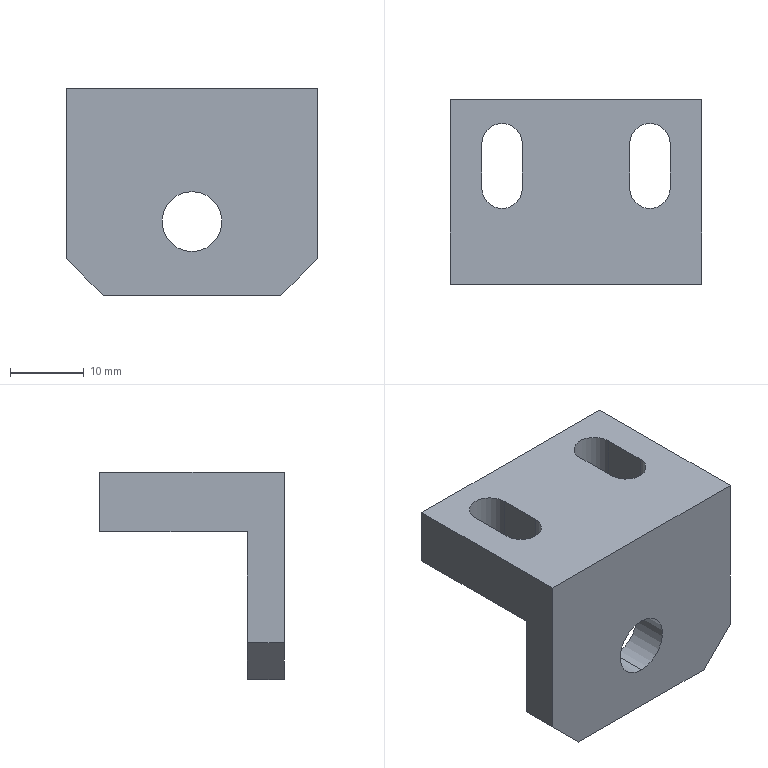Part | STEP file | push magnet cylinder seat | 1 solid | 20 faces | box 34 x 25 x 28 mm | volume 8909 mm3 | plane 14 | cylinder 6 | commonest cylinder face diameters 5.5 x4 8.1 x2